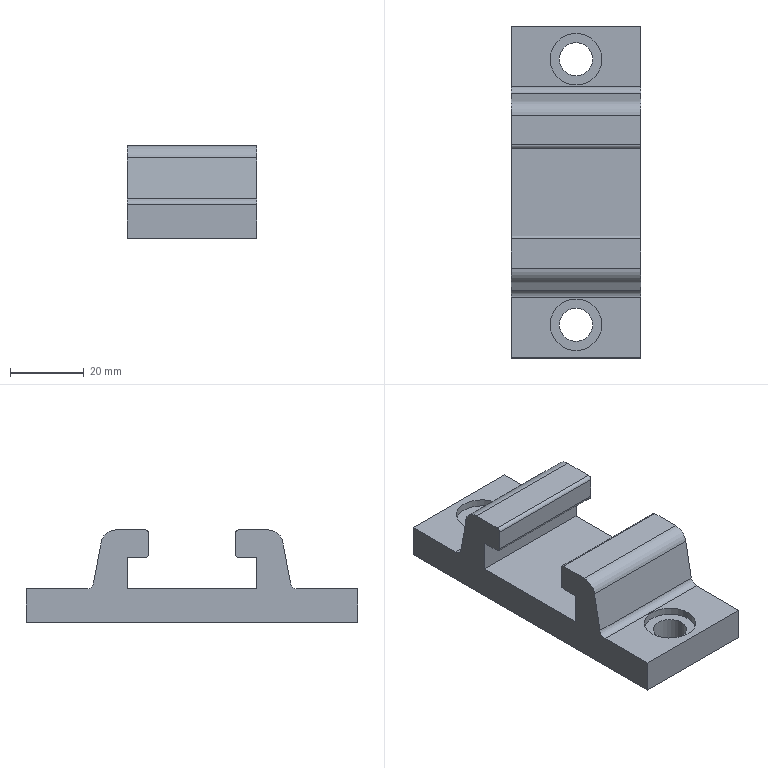Part | STEP file | YBQDJ-QD-8 | 1 solid | 32 faces | box 35 x 90 x 25 mm | volume 38677 mm3 | plane 20 | cylinder 12 | commonest cylinder face diameters 2 x4 4 x2 8 x2 9 x2 14 x2